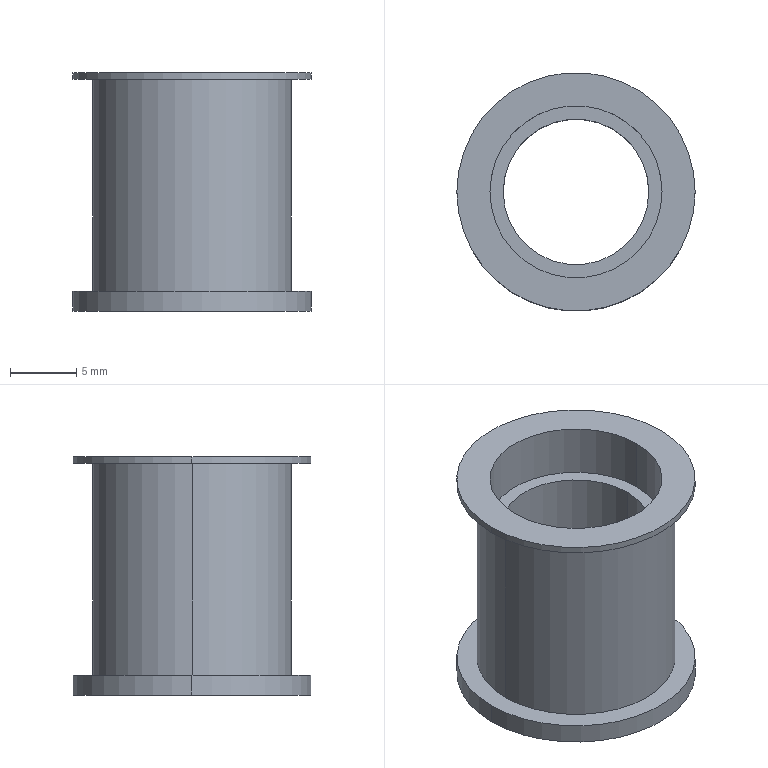Part | STEP file | 11-FG-SZ01011 | 1 solid | 18 faces | box 18 x 18 x 18 mm | volume 1437 mm3 | cylinder 12 | plane 6 | commonest cylinder face diameters 13 x4 18 x4 11 x2 15 x2
STEP:
#1=CARTESIAN_POINT('',(93.58,-247.716,1.));
#2=VERTEX_POINT('',#1);
#3=CARTESIAN_POINT('',(80.58,-247.716,1.));
#4=VERTEX_POINT('',#3);
#5=CARTESIAN_POINT('',(87.08,-247.716,1.));
#6=DIRECTION('',(0.,0.,-1.));
#7=DIRECTION('',(-1.,0.,0.));
#8=AXIS2_PLACEMENT_3D('',#5,#6,#7);
#9=CIRCLE('',#8,6.5);
#10=EDGE_CURVE('',#2,#4,#9,.T.);
#11=ORIENTED_EDGE('',*,*,#10,.F.);
#12=CARTESIAN_POINT('',(93.58,-247.716,0.));
#13=VERTEX_POINT('',#12);
#14=CARTESIAN_POINT('',(93.58,-247.716,1.));
#15=DIRECTION('',(0.,0.,-1.));
#16=VECTOR('',#15,1000.);
#17=LINE('',#14,#16);
#18=EDGE_CURVE('',#2,#13,#17,.T.);
#19=ORIENTED_EDGE('',*,*,#18,.T.);
#20=CARTESIAN_POINT('',(80.58,-247.716,0.));
#21=VERTEX_POINT('',#20);
#22=CARTESIAN_POINT('',(87.08,-247.716,0.));
#23=DIRECTION('',(0.,0.,-1.));
#24=DIRECTION('',(-1.,0.,0.));
#25=AXIS2_PLACEMENT_3D('',#22,#23,#24);
#26=CIRCLE('',#25,6.5);
#27=EDGE_CURVE('',#13,#21,#26,.T.);
#28=ORIENTED_EDGE('',*,*,#27,.T.);
#29=CARTESIAN_POINT('',(80.58,-247.716,1.));
#30=DIRECTION('',(0.,0.,-1.));
#31=VECTOR('',#30,1000.);
#32=LINE('',#29,#31);
#33=EDGE_CURVE('',#4,#21,#32,.T.);
#34=ORIENTED_EDGE('',*,*,#33,.F.);
#35=EDGE_LOOP('',(#11,#19,#28,#34));
#36=FACE_OUTER_BOUND('',#35,.T.);
#37=CARTESIAN_POINT('',(87.08,-247.716,1.));
#38=DIRECTION('',(0.,0.,-1.));
#39=DIRECTION('',(-1.,0.,0.));
#40=AXIS2_PLACEMENT_3D('',#37,#38,#39);
#41=CYLINDRICAL_SURFACE('',#40,6.5);
#42=ADVANCED_FACE('',(#36),#41,.F.);
#43=CARTESIAN_POINT('',(94.58,-247.716,1.5));
#44=VERTEX_POINT('',#43);
#45=CARTESIAN_POINT('',(79.58,-247.716,1.5));
#46=VERTEX_POINT('',#45);
#47=CARTESIAN_POINT('',(87.08,-247.716,1.5));
#48=DIRECTION('',(0.,0.,1.));
#49=DIRECTION('',(1.,0.,0.));
#50=AXIS2_PLACEMENT_3D('',#47,#48,#49);
#51=CIRCLE('',#50,7.5);
#52=EDGE_CURVE('',#44,#46,#51,.T.);
#53=ORIENTED_EDGE('',*,*,#52,.T.);
#54=CARTESIAN_POINT('',(79.58,-247.716,17.5));
#55=VERTEX_POINT('',#54);
#56=CARTESIAN_POINT('',(79.58,-247.716,1.5));
#57=DIRECTION('',(0.,0.,1.));
#58=VECTOR('',#57,1000.);
#59=LINE('',#56,#58);
#60=EDGE_CURVE('',#46,#55,#59,.T.);
#61=ORIENTED_EDGE('',*,*,#60,.T.);
#62=CARTESIAN_POINT('',(94.58,-247.716,17.5));
#63=VERTEX_POINT('',#62);
#64=CARTESIAN_POINT('',(87.08,-247.716,17.5));
#65=DIRECTION('',(0.,0.,1.));
#66=DIRECTION('',(1.,0.,0.));
#67=AXIS2_PLACEMENT_3D('',#64,#65,#66);
#68=CIRCLE('',#67,7.5);
#69=EDGE_CURVE('',#63,#55,#68,.T.);
#70=ORIENTED_EDGE('',*,*,#69,.F.);
#71=CARTESIAN_POINT('',(94.58,-247.716,1.5));
#72=DIRECTION('',(0.,0.,1.));
#73=VECTOR('',#72,1000.);
#74=LINE('',#71,#73);
#75=EDGE_CURVE('',#44,#63,#74,.T.);
#76=ORIENTED_EDGE('',*,*,#75,.F.);
#77=EDGE_LOOP('',(#53,#61,#70,#76));
#78=FACE_OUTER_BOUND('',#77,.T.);
#79=CARTESIAN_POINT('',(87.08,-247.716,1.5));
#80=DIRECTION('',(0.,0.,1.));
#81=DIRECTION('',(1.,0.,0.));
#82=AXIS2_PLACEMENT_3D('',#79,#80,#81);
#83=CYLINDRICAL_SURFACE('',#82,7.5);
#84=ADVANCED_FACE('',(#78),#83,.T.);
#85=CARTESIAN_POINT('',(96.08,-247.716,18.));
#86=VERTEX_POINT('',#85);
#87=CARTESIAN_POINT('',(78.08,-247.716,18.));
#88=VERTEX_POINT('',#87);
#89=CARTESIAN_POINT('',(87.08,-247.716,18.));
#90=DIRECTION('',(0.,0.,1.));
#91=DIRECTION('',(1.,0.,0.));
#92=AXIS2_PLACEMENT_3D('',#89,#90,#91);
#93=CIRCLE('',#92,9.);
#94=EDGE_CURVE('',#86,#88,#93,.T.);
#95=ORIENTED_EDGE('',*,*,#94,.F.);
#96=CARTESIAN_POINT('',(96.08,-247.716,17.5));
#97=VERTEX_POINT('',#96);
#98=CARTESIAN_POINT('',(96.08,-247.716,18.));
#99=DIRECTION('',(0.,0.,-1.));
#100=VECTOR('',#99,1000.);
#101=LINE('',#98,#100);
#102=EDGE_CURVE('',#86,#97,#101,.T.);
#103=ORIENTED_EDGE('',*,*,#102,.T.);
#104=CARTESIAN_POINT('',(78.08,-247.716,17.5));
#105=VERTEX_POINT('',#104);
#106=CARTESIAN_POINT('',(87.08,-247.716,17.5));
#107=DIRECTION('',(0.,0.,1.));
#108=DIRECTION('',(1.,0.,0.));
#109=AXIS2_PLACEMENT_3D('',#106,#107,#108);
#110=CIRCLE('',#109,9.);
#111=EDGE_CURVE('',#97,#105,#110,.T.);
#112=ORIENTED_EDGE('',*,*,#111,.T.);
#113=CARTESIAN_POINT('',(78.08,-247.716,18.));
#114=DIRECTION('',(0.,0.,-1.));
#115=VECTOR('',#114,1000.);
#116=LINE('',#113,#115);
#117=EDGE_CURVE('',#88,#105,#116,.T.);
#118=ORIENTED_EDGE('',*,*,#117,.F.);
#119=EDGE_LOOP('',(#95,#103,#112,#118));
#120=FACE_OUTER_BOUND('',#119,.T.);
#121=CARTESIAN_POINT('',(87.08,-247.716,18.));
#122=DIRECTION('',(0.,0.,-1.));
#123=DIRECTION('',(-1.,0.,0.));
#124=AXIS2_PLACEMENT_3D('',#121,#122,#123);
#125=CYLINDRICAL_SURFACE('',#124,9.);
#126=ADVANCED_FACE('',(#120),#125,.T.);
#127=CARTESIAN_POINT('',(80.58,-247.716,18.));
#128=VERTEX_POINT('',#127);
#129=CARTESIAN_POINT('',(93.58,-247.716,18.));
#130=VERTEX_POINT('',#129);
#131=CARTESIAN_POINT('',(87.08,-247.716,18.));
#132=DIRECTION('',(0.,0.,1.));
#133=DIRECTION('',(1.,0.,0.));
#134=AXIS2_PLACEMENT_3D('',#131,#132,#133);
#135=CIRCLE('',#134,6.5);
#136=EDGE_CURVE('',#128,#130,#135,.T.);
#137=ORIENTED_EDGE('',*,*,#136,.T.);
#138=CARTESIAN_POINT('',(93.58,-247.716,14.));
#139=VERTEX_POINT('',#138);
#140=CARTESIAN_POINT('',(93.58,-247.716,18.));
#141=DIRECTION('',(0.,0.,-1.));
#142=VECTOR('',#141,1000.);
#143=LINE('',#140,#142);
#144=EDGE_CURVE('',#130,#139,#143,.T.);
#145=ORIENTED_EDGE('',*,*,#144,.T.);
#146=CARTESIAN_POINT('',(80.58,-247.716,14.));
#147=VERTEX_POINT('',#146);
#148=CARTESIAN_POINT('',(87.08,-247.716,14.));
#149=DIRECTION('',(0.,0.,-1.));
#150=DIRECTION('',(-1.,0.,0.));
#151=AXIS2_PLACEMENT_3D('',#148,#149,#150);
#152=CIRCLE('',#151,6.5);
#153=EDGE_CURVE('',#139,#147,#152,.T.);
#154=ORIENTED_EDGE('',*,*,#153,.T.);
#155=CARTESIAN_POINT('',(80.58,-247.716,18.));
#156=DIRECTION('',(0.,0.,-1.));
#157=VECTOR('',#156,1000.);
#158=LINE('',#155,#157);
#159=EDGE_CURVE('',#128,#147,#158,.T.);
#160=ORIENTED_EDGE('',*,*,#159,.F.);
#161=EDGE_LOOP('',(#137,#145,#154,#160));
#162=FACE_OUTER_BOUND('',#161,.T.);
#163=CARTESIAN_POINT('',(87.08,-247.716,18.));
#164=DIRECTION('',(0.,0.,-1.));
#165=DIRECTION('',(-1.,0.,0.));
#166=AXIS2_PLACEMENT_3D('',#163,#164,#165);
#167=CYLINDRICAL_SURFACE('',#166,6.5);
#168=ADVANCED_FACE('',(#162),#167,.F.);
#169=CARTESIAN_POINT('',(96.08,-247.716,1.5));
#170=VERTEX_POINT('',#169);
#171=CARTESIAN_POINT('',(78.08,-247.716,1.5));
#172=VERTEX_POINT('',#171);
#173=CARTESIAN_POINT('',(87.08,-247.716,1.5));
#174=DIRECTION('',(0.,0.,1.));
#175=DIRECTION('',(1.,0.,0.));
#176=AXIS2_PLACEMENT_3D('',#173,#174,#175);
#177=CIRCLE('',#176,9.);
#178=EDGE_CURVE('',#170,#172,#177,.T.);
#179=ORIENTED_EDGE('',*,*,#178,.F.);
#180=CARTESIAN_POINT('',(96.08,-247.716,0.));
#181=VERTEX_POINT('',#180);
#182=CARTESIAN_POINT('',(96.08,-247.716,18.));
#183=DIRECTION('',(0.,0.,-1.));
#184=VECTOR('',#183,1000.);
#185=LINE('',#182,#184);
#186=EDGE_CURVE('',#170,#181,#185,.T.);
#187=ORIENTED_EDGE('',*,*,#186,.T.);
#188=CARTESIAN_POINT('',(78.08,-247.716,0.));
#189=VERTEX_POINT('',#188);
#190=CARTESIAN_POINT('',(87.08,-247.716,0.));
#191=DIRECTION('',(0.,0.,1.));
#192=DIRECTION('',(1.,0.,0.));
#193=AXIS2_PLACEMENT_3D('',#190,#191,#192);
#194=CIRCLE('',#193,9.);
#195=EDGE_CURVE('',#181,#189,#194,.T.);
#196=ORIENTED_EDGE('',*,*,#195,.T.);
#197=CARTESIAN_POINT('',(78.08,-247.716,18.));
#198=DIRECTION('',(0.,0.,-1.));
#199=VECTOR('',#198,1000.);
#200=LINE('',#197,#199);
#201=EDGE_CURVE('',#172,#189,#200,.T.);
#202=ORIENTED_EDGE('',*,*,#201,.F.);
#203=EDGE_LOOP('',(#179,#187,#196,#202));
#204=FACE_OUTER_BOUND('',#203,.T.);
#205=CARTESIAN_POINT('',(87.08,-247.716,18.));
#206=DIRECTION('',(0.,0.,-1.));
#207=DIRECTION('',(-1.,0.,0.));
#208=AXIS2_PLACEMENT_3D('',#205,#206,#207);
#209=CYLINDRICAL_SURFACE('',#208,9.);
#210=ADVANCED_FACE('',(#204),#209,.T.);
#211=CARTESIAN_POINT('',(92.58,-247.716,14.));
#212=VERTEX_POINT('',#211);
#213=CARTESIAN_POINT('',(81.58,-247.716,14.));
#214=VERTEX_POINT('',#213);
#215=CARTESIAN_POINT('',(87.08,-247.716,14.));
#216=DIRECTION('',(0.,0.,-1.));
#217=DIRECTION('',(-1.,0.,0.));
#218=AXIS2_PLACEMENT_3D('',#215,#216,#217);
#219=CIRCLE('',#218,5.5);
#220=EDGE_CURVE('',#212,#214,#219,.T.);
#221=ORIENTED_EDGE('',*,*,#220,.F.);
#222=CARTESIAN_POINT('',(92.58,-247.716,1.));
#223=VERTEX_POINT('',#222);
#224=CARTESIAN_POINT('',(92.58,-247.716,14.));
#225=DIRECTION('',(0.,0.,-1.));
#226=VECTOR('',#225,1000.);
#227=LINE('',#224,#226);
#228=EDGE_CURVE('',#212,#223,#227,.T.);
#229=ORIENTED_EDGE('',*,*,#228,.T.);
#230=CARTESIAN_POINT('',(81.58,-247.716,1.));
#231=VERTEX_POINT('',#230);
#232=CARTESIAN_POINT('',(87.08,-247.716,1.));
#233=DIRECTION('',(0.,0.,1.));
#234=DIRECTION('',(-1.,0.,0.));
#235=AXIS2_PLACEMENT_3D('',#232,#233,#234);
#236=CIRCLE('',#235,5.5);
#237=EDGE_CURVE('',#231,#223,#236,.T.);
#238=ORIENTED_EDGE('',*,*,#237,.F.);
#239=CARTESIAN_POINT('',(81.58,-247.716,14.));
#240=DIRECTION('',(0.,0.,-1.));
#241=VECTOR('',#240,1000.);
#242=LINE('',#239,#241);
#243=EDGE_CURVE('',#214,#231,#242,.T.);
#244=ORIENTED_EDGE('',*,*,#243,.F.);
#245=EDGE_LOOP('',(#221,#229,#238,#244));
#246=FACE_OUTER_BOUND('',#245,.T.);
#247=CARTESIAN_POINT('',(87.08,-247.716,14.));
#248=DIRECTION('',(0.,0.,-1.));
#249=DIRECTION('',(-1.,0.,0.));
#250=AXIS2_PLACEMENT_3D('',#247,#248,#249);
#251=CYLINDRICAL_SURFACE('',#250,5.5);
#252=ADVANCED_FACE('',(#246),#251,.F.);
#253=ORIENTED_EDGE('',*,*,#228,.F.);
#254=CARTESIAN_POINT('',(87.08,-247.716,14.));
#255=DIRECTION('',(0.,0.,-1.));
#256=DIRECTION('',(-1.,0.,0.));
#257=AXIS2_PLACEMENT_3D('',#254,#255,#256);
#258=CIRCLE('',#257,5.5);
#259=EDGE_CURVE('',#214,#212,#258,.T.);
#260=ORIENTED_EDGE('',*,*,#259,.F.);
#261=ORIENTED_EDGE('',*,*,#243,.T.);
#262=CARTESIAN_POINT('',(87.08,-247.716,1.));
#263=DIRECTION('',(0.,0.,1.));
#264=DIRECTION('',(-1.,0.,0.));
#265=AXIS2_PLACEMENT_3D('',#262,#263,#264);
#266=CIRCLE('',#265,5.5);
#267=EDGE_CURVE('',#223,#231,#266,.T.);
#268=ORIENTED_EDGE('',*,*,#267,.F.);
#269=EDGE_LOOP('',(#253,#260,#261,#268));
#270=FACE_OUTER_BOUND('',#269,.T.);
#271=CARTESIAN_POINT('',(87.08,-247.716,14.));
#272=DIRECTION('',(0.,0.,-1.));
#273=DIRECTION('',(-1.,0.,0.));
#274=AXIS2_PLACEMENT_3D('',#271,#272,#273);
#275=CYLINDRICAL_SURFACE('',#274,5.5);
#276=ADVANCED_FACE('',(#270),#275,.F.);
#277=ORIENTED_EDGE('',*,*,#186,.F.);
#278=CARTESIAN_POINT('',(87.08,-247.716,1.5));
#279=DIRECTION('',(0.,0.,1.));
#280=DIRECTION('',(1.,0.,0.));
#281=AXIS2_PLACEMENT_3D('',#278,#279,#280);
#282=CIRCLE('',#281,9.);
#283=EDGE_CURVE('',#172,#170,#282,.T.);
#284=ORIENTED_EDGE('',*,*,#283,.F.);
#285=ORIENTED_EDGE('',*,*,#201,.T.);
#286=CARTESIAN_POINT('',(87.08,-247.716,0.));
#287=DIRECTION('',(0.,0.,1.));
#288=DIRECTION('',(1.,0.,0.));
#289=AXIS2_PLACEMENT_3D('',#286,#287,#288);
#290=CIRCLE('',#289,9.);
#291=EDGE_CURVE('',#189,#181,#290,.T.);
#292=ORIENTED_EDGE('',*,*,#291,.T.);
#293=EDGE_LOOP('',(#277,#284,#285,#292));
#294=FACE_OUTER_BOUND('',#293,.T.);
#295=CARTESIAN_POINT('',(87.08,-247.716,18.));
#296=DIRECTION('',(0.,0.,-1.));
#297=DIRECTION('',(-1.,0.,0.));
#298=AXIS2_PLACEMENT_3D('',#295,#296,#297);
#299=CYLINDRICAL_SURFACE('',#298,9.);
#300=ADVANCED_FACE('',(#294),#299,.T.);
#301=ORIENTED_EDGE('',*,*,#144,.F.);
#302=CARTESIAN_POINT('',(87.08,-247.716,18.));
#303=DIRECTION('',(0.,0.,1.));
#304=DIRECTION('',(1.,0.,0.));
#305=AXIS2_PLACEMENT_3D('',#302,#303,#304);
#306=CIRCLE('',#305,6.5);
#307=EDGE_CURVE('',#130,#128,#306,.T.);
#308=ORIENTED_EDGE('',*,*,#307,.T.);
#309=ORIENTED_EDGE('',*,*,#159,.T.);
#310=CARTESIAN_POINT('',(87.08,-247.716,14.));
#311=DIRECTION('',(0.,0.,-1.));
#312=DIRECTION('',(-1.,0.,0.));
#313=AXIS2_PLACEMENT_3D('',#310,#311,#312);
#314=CIRCLE('',#313,6.5);
#315=EDGE_CURVE('',#147,#139,#314,.T.);
#316=ORIENTED_EDGE('',*,*,#315,.T.);
#317=EDGE_LOOP('',(#301,#308,#309,#316));
#318=FACE_OUTER_BOUND('',#317,.T.);
#319=CARTESIAN_POINT('',(87.08,-247.716,18.));
#320=DIRECTION('',(0.,0.,-1.));
#321=DIRECTION('',(-1.,0.,0.));
#322=AXIS2_PLACEMENT_3D('',#319,#320,#321);
#323=CYLINDRICAL_SURFACE('',#322,6.5);
#324=ADVANCED_FACE('',(#318),#323,.F.);
#325=CARTESIAN_POINT('',(87.08,-247.716,18.));
#326=DIRECTION('',(0.,0.,1.));
#327=DIRECTION('',(1.,0.,0.));
#328=AXIS2_PLACEMENT_3D('',#325,#326,#327);
#329=CIRCLE('',#328,9.);
#330=EDGE_CURVE('',#88,#86,#329,.T.);
#331=ORIENTED_EDGE('',*,*,#330,.T.);
#332=ORIENTED_EDGE('',*,*,#94,.T.);
#333=EDGE_LOOP('',(#331,#332));
#334=FACE_OUTER_BOUND('',#333,.T.);
#335=ORIENTED_EDGE('',*,*,#136,.F.);
#336=ORIENTED_EDGE('',*,*,#307,.F.);
#337=EDGE_LOOP('',(#335,#336));
#338=FACE_BOUND('',#337,.T.);
#339=CARTESIAN_POINT('',(87.08,-247.716,18.));
#340=DIRECTION('',(0.,0.,1.));
#341=DIRECTION('',(1.,0.,0.));
#342=AXIS2_PLACEMENT_3D('',#339,#340,#341);
#343=PLANE('',#342);
#344=ADVANCED_FACE('',(#334,#338),#343,.T.);
#345=CARTESIAN_POINT('',(87.08,-247.716,0.));
#346=DIRECTION('',(0.,0.,-1.));
#347=DIRECTION('',(-1.,0.,0.));
#348=AXIS2_PLACEMENT_3D('',#345,#346,#347);
#349=CIRCLE('',#348,6.5);
#350=EDGE_CURVE('',#21,#13,#349,.T.);
#351=ORIENTED_EDGE('',*,*,#350,.F.);
#352=ORIENTED_EDGE('',*,*,#27,.F.);
#353=EDGE_LOOP('',(#351,#352));
#354=FACE_BOUND('',#353,.T.);
#355=ORIENTED_EDGE('',*,*,#291,.F.);
#356=ORIENTED_EDGE('',*,*,#195,.F.);
#357=EDGE_LOOP('',(#355,#356));
#358=FACE_OUTER_BOUND('',#357,.T.);
#359=CARTESIAN_POINT('',(87.08,-247.716,0.));
#360=DIRECTION('',(0.,0.,1.));
#361=DIRECTION('',(1.,0.,0.));
#362=AXIS2_PLACEMENT_3D('',#359,#360,#361);
#363=PLANE('',#362);
#364=ADVANCED_FACE('',(#354,#358),#363,.F.);
#365=ORIENTED_EDGE('',*,*,#102,.F.);
#366=ORIENTED_EDGE('',*,*,#330,.F.);
#367=ORIENTED_EDGE('',*,*,#117,.T.);
#368=CARTESIAN_POINT('',(87.08,-247.716,17.5));
#369=DIRECTION('',(0.,0.,1.));
#370=DIRECTION('',(1.,0.,0.));
#371=AXIS2_PLACEMENT_3D('',#368,#369,#370);
#372=CIRCLE('',#371,9.);
#373=EDGE_CURVE('',#105,#97,#372,.T.);
#374=ORIENTED_EDGE('',*,*,#373,.T.);
#375=EDGE_LOOP('',(#365,#366,#367,#374));
#376=FACE_OUTER_BOUND('',#375,.T.);
#377=CARTESIAN_POINT('',(87.08,-247.716,18.));
#378=DIRECTION('',(0.,0.,-1.));
#379=DIRECTION('',(-1.,0.,0.));
#380=AXIS2_PLACEMENT_3D('',#377,#378,#379);
#381=CYLINDRICAL_SURFACE('',#380,9.);
#382=ADVANCED_FACE('',(#376),#381,.T.);
#383=ORIENTED_EDGE('',*,*,#259,.T.);
#384=ORIENTED_EDGE('',*,*,#220,.T.);
#385=EDGE_LOOP('',(#383,#384));
#386=FACE_BOUND('',#385,.T.);
#387=ORIENTED_EDGE('',*,*,#315,.F.);
#388=ORIENTED_EDGE('',*,*,#153,.F.);
#389=EDGE_LOOP('',(#387,#388));
#390=FACE_OUTER_BOUND('',#389,.T.);
#391=CARTESIAN_POINT('',(87.08,-247.716,14.));
#392=DIRECTION('',(0.,0.,-1.));
#393=DIRECTION('',(-1.,0.,0.));
#394=AXIS2_PLACEMENT_3D('',#391,#392,#393);
#395=PLANE('',#394);
#396=ADVANCED_FACE('',(#386,#390),#395,.F.);
#397=ORIENTED_EDGE('',*,*,#52,.F.);
#398=CARTESIAN_POINT('',(87.08,-247.716,1.5));
#399=DIRECTION('',(0.,0.,1.));
#400=DIRECTION('',(1.,0.,0.));
#401=AXIS2_PLACEMENT_3D('',#398,#399,#400);
#402=CIRCLE('',#401,7.5);
#403=EDGE_CURVE('',#46,#44,#402,.T.);
#404=ORIENTED_EDGE('',*,*,#403,.F.);
#405=EDGE_LOOP('',(#397,#404));
#406=FACE_BOUND('',#405,.T.);
#407=ORIENTED_EDGE('',*,*,#283,.T.);
#408=ORIENTED_EDGE('',*,*,#178,.T.);
#409=EDGE_LOOP('',(#407,#408));
#410=FACE_OUTER_BOUND('',#409,.T.);
#411=CARTESIAN_POINT('',(87.08,-247.716,1.5));
#412=DIRECTION('',(0.,0.,1.));
#413=DIRECTION('',(1.,0.,0.));
#414=AXIS2_PLACEMENT_3D('',#411,#412,#413);
#415=PLANE('',#414);
#416=ADVANCED_FACE('',(#406,#410),#415,.T.);
#417=ORIENTED_EDGE('',*,*,#69,.T.);
#418=CARTESIAN_POINT('',(87.08,-247.716,17.5));
#419=DIRECTION('',(0.,0.,1.));
#420=DIRECTION('',(1.,0.,0.));
#421=AXIS2_PLACEMENT_3D('',#418,#419,#420);
#422=CIRCLE('',#421,7.5);
#423=EDGE_CURVE('',#55,#63,#422,.T.);
#424=ORIENTED_EDGE('',*,*,#423,.T.);
#425=EDGE_LOOP('',(#417,#424));
#426=FACE_BOUND('',#425,.T.);
#427=ORIENTED_EDGE('',*,*,#373,.F.);
#428=ORIENTED_EDGE('',*,*,#111,.F.);
#429=EDGE_LOOP('',(#427,#428));
#430=FACE_OUTER_BOUND('',#429,.T.);
#431=CARTESIAN_POINT('',(87.08,-247.716,17.5));
#432=DIRECTION('',(0.,0.,1.));
#433=DIRECTION('',(1.,0.,0.));
#434=AXIS2_PLACEMENT_3D('',#431,#432,#433);
#435=PLANE('',#434);
#436=ADVANCED_FACE('',(#426,#430),#435,.F.);
#437=ORIENTED_EDGE('',*,*,#60,.F.);
#438=ORIENTED_EDGE('',*,*,#403,.T.);
#439=ORIENTED_EDGE('',*,*,#75,.T.);
#440=ORIENTED_EDGE('',*,*,#423,.F.);
#441=EDGE_LOOP('',(#437,#438,#439,#440));
#442=FACE_OUTER_BOUND('',#441,.T.);
#443=CARTESIAN_POINT('',(87.08,-247.716,1.5));
#444=DIRECTION('',(0.,0.,1.));
#445=DIRECTION('',(1.,0.,0.));
#446=AXIS2_PLACEMENT_3D('',#443,#444,#445);
#447=CYLINDRICAL_SURFACE('',#446,7.5);
#448=ADVANCED_FACE('',(#442),#447,.T.);
#449=CARTESIAN_POINT('',(87.08,-247.716,1.));
#450=DIRECTION('',(0.,0.,-1.));
#451=DIRECTION('',(-1.,0.,0.));
#452=AXIS2_PLACEMENT_3D('',#449,#450,#451);
#453=CIRCLE('',#452,6.5);
#454=EDGE_CURVE('',#4,#2,#453,.T.);
#455=ORIENTED_EDGE('',*,*,#454,.T.);
#456=ORIENTED_EDGE('',*,*,#10,.T.);
#457=EDGE_LOOP('',(#455,#456));
#458=FACE_OUTER_BOUND('',#457,.T.);
#459=ORIENTED_EDGE('',*,*,#237,.T.);
#460=ORIENTED_EDGE('',*,*,#267,.T.);
#461=EDGE_LOOP('',(#459,#460));
#462=FACE_BOUND('',#461,.T.);
#463=CARTESIAN_POINT('',(87.08,-247.716,1.));
#464=DIRECTION('',(0.,0.,-1.));
#465=DIRECTION('',(-1.,0.,0.));
#466=AXIS2_PLACEMENT_3D('',#463,#464,#465);
#467=PLANE('',#466);
#468=ADVANCED_FACE('',(#458,#462),#467,.T.);
#469=ORIENTED_EDGE('',*,*,#18,.F.);
#470=ORIENTED_EDGE('',*,*,#454,.F.);
#471=ORIENTED_EDGE('',*,*,#33,.T.);
#472=ORIENTED_EDGE('',*,*,#350,.T.);
#473=EDGE_LOOP('',(#469,#470,#471,#472));
#474=FACE_OUTER_BOUND('',#473,.T.);
#475=CARTESIAN_POINT('',(87.08,-247.716,1.));
#476=DIRECTION('',(0.,0.,-1.));
#477=DIRECTION('',(-1.,0.,0.));
#478=AXIS2_PLACEMENT_3D('',#475,#476,#477);
#479=CYLINDRICAL_SURFACE('',#478,6.5);
#480=ADVANCED_FACE('',(#474),#479,.F.);
#481=CLOSED_SHELL('',(#42,#84,#126,#168,#210,#252,#276,#300,#324,#344,#364,#382,#396,#416,#436,#448,#468,#480));
#482=MANIFOLD_SOLID_BREP('',#481);
#483=CARTESIAN_POINT('',(0.,0.,0.));
#484=DIRECTION('',(0.,0.,1.));
#485=DIRECTION('',(1.,0.,0.));
#486=AXIS2_PLACEMENT_3D('',#483,#484,#485);
#487=(LENGTH_UNIT()NAMED_UNIT(*)SI_UNIT(.MILLI.,.METRE.));
#488=UNCERTAINTY_MEASURE_WITH_UNIT(LENGTH_MEASURE(0.00001),#487,'','');
#489=(NAMED_UNIT(*)PLANE_ANGLE_UNIT()SI_UNIT($,.RADIAN.));
#490=(NAMED_UNIT(*)SI_UNIT($,.STERADIAN.)SOLID_ANGLE_UNIT());
#491=(GEOMETRIC_REPRESENTATION_CONTEXT(3)GLOBAL_UNCERTAINTY_ASSIGNED_CONTEXT((#488))GLOBAL_UNIT_ASSIGNED_CONTEXT((#487,#489,#490))REPRESENTATION_CONTEXT('',''));
#492=ADVANCED_BREP_SHAPE_REPRESENTATION('',(#482,#486),#491);